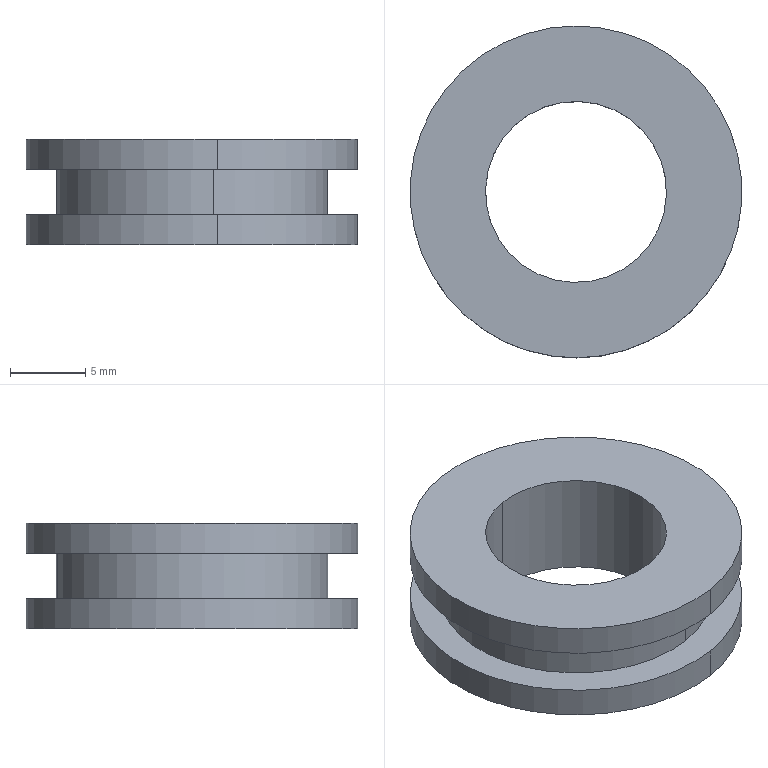Part | SolidWorks | features BaseBody 1 | 1 solid | 12 faces | box 22.001 x 22 x 7.003 mm | volume 1492 mm3 | cylinder 8 | plane 4 | commonest cylinder face diameters 22 x4 12 x2 18 x2
STEP:
#1=CARTESIAN_POINT('',(416.566,223.384,18.485));
#2=VERTEX_POINT('',#1);
#3=CARTESIAN_POINT('',(419.971,201.649,18.486));
#4=VERTEX_POINT('',#3);
#5=CARTESIAN_POINT('',(418.268,212.516,18.486));
#6=DIRECTION('',(0.0001435,0.000000521,-1.));
#7=DIRECTION('',(-0.1548,0.988,-0.00002169));
#8=AXIS2_PLACEMENT_3D('',#5,#6,#7);
#9=CIRCLE('',#8,11.);
#10=EDGE_CURVE('',#2,#4,#9,.T.);
#11=ORIENTED_EDGE('',*,*,#10,.F.);
#12=CARTESIAN_POINT('',(416.565,223.384,20.485));
#13=VERTEX_POINT('',#12);
#14=CARTESIAN_POINT('',(416.566,223.384,13.485));
#15=DIRECTION('',(-0.0001435,-0.000000521,1.));
#16=VECTOR('',#15,1000.);
#17=LINE('',#14,#16);
#18=EDGE_CURVE('',#2,#13,#17,.T.);
#19=ORIENTED_EDGE('',*,*,#18,.T.);
#20=CARTESIAN_POINT('',(419.97,201.649,20.486));
#21=VERTEX_POINT('',#20);
#22=CARTESIAN_POINT('',(418.268,212.516,20.486));
#23=DIRECTION('',(-0.0001435,-0.000000521,1.));
#24=DIRECTION('',(0.1548,-0.988,0.00002169));
#25=AXIS2_PLACEMENT_3D('',#22,#23,#24);
#26=CIRCLE('',#25,11.);
#27=EDGE_CURVE('',#21,#13,#26,.T.);
#28=ORIENTED_EDGE('',*,*,#27,.F.);
#29=CARTESIAN_POINT('',(419.971,201.649,13.486));
#30=DIRECTION('',(-0.0001435,-0.000000521,1.));
#31=VECTOR('',#30,1000.);
#32=LINE('',#29,#31);
#33=EDGE_CURVE('',#4,#21,#32,.T.);
#34=ORIENTED_EDGE('',*,*,#33,.F.);
#35=EDGE_LOOP('',(#11,#19,#28,#34));
#36=FACE_OUTER_BOUND('',#35,.T.);
#37=CARTESIAN_POINT('',(418.269,212.516,13.486));
#38=DIRECTION('',(-0.0001435,-0.000000521,1.));
#39=DIRECTION('',(0.1548,-0.988,0.00002169));
#40=AXIS2_PLACEMENT_3D('',#37,#38,#39);
#41=CYLINDRICAL_SURFACE('',#40,11.);
#42=ADVANCED_FACE('',(#36),#41,.T.);
#43=CARTESIAN_POINT('',(419.661,203.625,18.486));
#44=VERTEX_POINT('',#43);
#45=CARTESIAN_POINT('',(416.875,221.408,18.485));
#46=VERTEX_POINT('',#45);
#47=CARTESIAN_POINT('',(418.268,212.516,18.486));
#48=DIRECTION('',(-0.0001435,-0.000000521,1.));
#49=DIRECTION('',(0.1548,-0.988,0.00002169));
#50=AXIS2_PLACEMENT_3D('',#47,#48,#49);
#51=CIRCLE('',#50,9.);
#52=EDGE_CURVE('',#44,#46,#51,.T.);
#53=ORIENTED_EDGE('',*,*,#52,.F.);
#54=CARTESIAN_POINT('',(419.662,203.625,15.486));
#55=VERTEX_POINT('',#54);
#56=CARTESIAN_POINT('',(419.661,203.625,19.486));
#57=DIRECTION('',(0.0001435,0.000000521,-1.));
#58=VECTOR('',#57,1000.);
#59=LINE('',#56,#58);
#60=EDGE_CURVE('',#44,#55,#59,.T.);
#61=ORIENTED_EDGE('',*,*,#60,.T.);
#62=CARTESIAN_POINT('',(416.876,221.408,15.485));
#63=VERTEX_POINT('',#62);
#64=CARTESIAN_POINT('',(418.269,212.516,15.486));
#65=DIRECTION('',(0.0001435,0.000000521,-1.));
#66=DIRECTION('',(0.1548,-0.988,0.00002169));
#67=AXIS2_PLACEMENT_3D('',#64,#65,#66);
#68=CIRCLE('',#67,9.);
#69=EDGE_CURVE('',#63,#55,#68,.T.);
#70=ORIENTED_EDGE('',*,*,#69,.F.);
#71=CARTESIAN_POINT('',(416.875,221.408,19.485));
#72=DIRECTION('',(0.0001435,0.000000521,-1.));
#73=VECTOR('',#72,1000.);
#74=LINE('',#71,#73);
#75=EDGE_CURVE('',#46,#63,#74,.T.);
#76=ORIENTED_EDGE('',*,*,#75,.F.);
#77=EDGE_LOOP('',(#53,#61,#70,#76));
#78=FACE_OUTER_BOUND('',#77,.T.);
#79=CARTESIAN_POINT('',(418.268,212.516,19.486));
#80=DIRECTION('',(0.0001435,0.000000521,-1.));
#81=DIRECTION('',(-0.1548,0.988,-0.00002169));
#82=AXIS2_PLACEMENT_3D('',#79,#80,#81);
#83=CYLINDRICAL_SURFACE('',#82,9.);
#84=ADVANCED_FACE('',(#78),#83,.T.);
#85=CARTESIAN_POINT('',(416.566,223.384,13.485));
#86=VERTEX_POINT('',#85);
#87=CARTESIAN_POINT('',(419.971,201.649,13.486));
#88=VERTEX_POINT('',#87);
#89=CARTESIAN_POINT('',(418.269,212.516,13.486));
#90=DIRECTION('',(0.0001435,0.000000521,-1.));
#91=DIRECTION('',(1.,0.,0.0001435));
#92=AXIS2_PLACEMENT_3D('',#89,#90,#91);
#93=CIRCLE('',#92,11.);
#94=EDGE_CURVE('',#86,#88,#93,.T.);
#95=ORIENTED_EDGE('',*,*,#94,.F.);
#96=CARTESIAN_POINT('',(416.566,223.384,15.485));
#97=VERTEX_POINT('',#96);
#98=CARTESIAN_POINT('',(416.566,223.384,13.485));
#99=DIRECTION('',(-0.0001435,-0.000000521,1.));
#100=VECTOR('',#99,1000.);
#101=LINE('',#98,#100);
#102=EDGE_CURVE('',#86,#97,#101,.T.);
#103=ORIENTED_EDGE('',*,*,#102,.T.);
#104=CARTESIAN_POINT('',(419.971,201.649,15.486));
#105=VERTEX_POINT('',#104);
#106=CARTESIAN_POINT('',(418.269,212.516,15.486));
#107=DIRECTION('',(-0.0001435,-0.000000521,1.));
#108=DIRECTION('',(-0.1548,0.988,-0.00002169));
#109=AXIS2_PLACEMENT_3D('',#106,#107,#108);
#110=CIRCLE('',#109,11.);
#111=EDGE_CURVE('',#105,#97,#110,.T.);
#112=ORIENTED_EDGE('',*,*,#111,.F.);
#113=CARTESIAN_POINT('',(419.971,201.649,13.486));
#114=DIRECTION('',(-0.0001435,-0.000000521,1.));
#115=VECTOR('',#114,1000.);
#116=LINE('',#113,#115);
#117=EDGE_CURVE('',#88,#105,#116,.T.);
#118=ORIENTED_EDGE('',*,*,#117,.F.);
#119=EDGE_LOOP('',(#95,#103,#112,#118));
#120=FACE_OUTER_BOUND('',#119,.T.);
#121=CARTESIAN_POINT('',(418.269,212.516,13.486));
#122=DIRECTION('',(-0.0001435,-0.000000521,1.));
#123=DIRECTION('',(0.1548,-0.988,0.00002169));
#124=AXIS2_PLACEMENT_3D('',#121,#122,#123);
#125=CYLINDRICAL_SURFACE('',#124,11.);
#126=ADVANCED_FACE('',(#120),#125,.T.);
#127=CARTESIAN_POINT('',(419.196,206.589,20.486));
#128=VERTEX_POINT('',#127);
#129=CARTESIAN_POINT('',(417.339,218.444,20.485));
#130=VERTEX_POINT('',#129);
#131=CARTESIAN_POINT('',(418.268,212.516,20.486));
#132=DIRECTION('',(0.0001435,0.000000521,-1.));
#133=DIRECTION('',(-1.,0.,-0.0001435));
#134=AXIS2_PLACEMENT_3D('',#131,#132,#133);
#135=CIRCLE('',#134,6.);
#136=EDGE_CURVE('',#128,#130,#135,.T.);
#137=ORIENTED_EDGE('',*,*,#136,.F.);
#138=CARTESIAN_POINT('',(419.197,206.589,13.486));
#139=VERTEX_POINT('',#138);
#140=CARTESIAN_POINT('',(419.197,206.589,19.486));
#141=DIRECTION('',(0.0001435,0.000000521,-1.));
#142=VECTOR('',#141,1000.);
#143=LINE('',#140,#142);
#144=EDGE_CURVE('',#128,#139,#143,.T.);
#145=ORIENTED_EDGE('',*,*,#144,.T.);
#146=CARTESIAN_POINT('',(417.34,218.444,13.485));
#147=VERTEX_POINT('',#146);
#148=CARTESIAN_POINT('',(418.269,212.516,13.486));
#149=DIRECTION('',(-0.0001435,-0.000000521,1.));
#150=DIRECTION('',(0.1548,-0.988,0.00002169));
#151=AXIS2_PLACEMENT_3D('',#148,#149,#150);
#152=CIRCLE('',#151,6.);
#153=EDGE_CURVE('',#147,#139,#152,.T.);
#154=ORIENTED_EDGE('',*,*,#153,.F.);
#155=CARTESIAN_POINT('',(417.339,218.444,19.485));
#156=DIRECTION('',(0.0001435,0.000000521,-1.));
#157=VECTOR('',#156,1000.);
#158=LINE('',#155,#157);
#159=EDGE_CURVE('',#130,#147,#158,.T.);
#160=ORIENTED_EDGE('',*,*,#159,.F.);
#161=EDGE_LOOP('',(#137,#145,#154,#160));
#162=FACE_OUTER_BOUND('',#161,.T.);
#163=CARTESIAN_POINT('',(418.268,212.516,19.486));
#164=DIRECTION('',(0.0001435,0.000000521,-1.));
#165=DIRECTION('',(-0.1548,0.988,-0.00002169));
#166=AXIS2_PLACEMENT_3D('',#163,#164,#165);
#167=CYLINDRICAL_SURFACE('',#166,6.);
#168=ADVANCED_FACE('',(#162),#167,.F.);
#169=CARTESIAN_POINT('',(418.268,212.516,20.486));
#170=DIRECTION('',(0.0001435,0.000000521,-1.));
#171=DIRECTION('',(-1.,0.,-0.0001435));
#172=AXIS2_PLACEMENT_3D('',#169,#170,#171);
#173=CIRCLE('',#172,6.);
#174=EDGE_CURVE('',#130,#128,#173,.T.);
#175=ORIENTED_EDGE('',*,*,#174,.T.);
#176=ORIENTED_EDGE('',*,*,#136,.T.);
#177=EDGE_LOOP('',(#175,#176));
#178=FACE_BOUND('',#177,.T.);
#179=ORIENTED_EDGE('',*,*,#27,.T.);
#180=CARTESIAN_POINT('',(418.268,212.516,20.486));
#181=DIRECTION('',(-0.0001435,-0.000000521,1.));
#182=DIRECTION('',(0.1548,-0.988,0.00002169));
#183=AXIS2_PLACEMENT_3D('',#180,#181,#182);
#184=CIRCLE('',#183,11.);
#185=EDGE_CURVE('',#13,#21,#184,.T.);
#186=ORIENTED_EDGE('',*,*,#185,.T.);
#187=EDGE_LOOP('',(#179,#186));
#188=FACE_OUTER_BOUND('',#187,.T.);
#189=CARTESIAN_POINT('',(418.268,212.516,20.486));
#190=DIRECTION('',(-0.0001435,-0.000000521,1.));
#191=DIRECTION('',(-0.003633,1.,0.));
#192=AXIS2_PLACEMENT_3D('',#189,#190,#191);
#193=PLANE('',#192);
#194=ADVANCED_FACE('',(#178,#188),#193,.T.);
#195=ORIENTED_EDGE('',*,*,#144,.F.);
#196=ORIENTED_EDGE('',*,*,#174,.F.);
#197=ORIENTED_EDGE('',*,*,#159,.T.);
#198=CARTESIAN_POINT('',(418.269,212.516,13.486));
#199=DIRECTION('',(-0.0001435,-0.000000521,1.));
#200=DIRECTION('',(0.1548,-0.988,0.00002169));
#201=AXIS2_PLACEMENT_3D('',#198,#199,#200);
#202=CIRCLE('',#201,6.);
#203=EDGE_CURVE('',#139,#147,#202,.T.);
#204=ORIENTED_EDGE('',*,*,#203,.F.);
#205=EDGE_LOOP('',(#195,#196,#197,#204));
#206=FACE_OUTER_BOUND('',#205,.T.);
#207=CARTESIAN_POINT('',(418.268,212.516,19.486));
#208=DIRECTION('',(0.0001435,0.000000521,-1.));
#209=DIRECTION('',(-0.1548,0.988,-0.00002169));
#210=AXIS2_PLACEMENT_3D('',#207,#208,#209);
#211=CYLINDRICAL_SURFACE('',#210,6.);
#212=ADVANCED_FACE('',(#206),#211,.F.);
#213=ORIENTED_EDGE('',*,*,#153,.T.);
#214=ORIENTED_EDGE('',*,*,#203,.T.);
#215=EDGE_LOOP('',(#213,#214));
#216=FACE_BOUND('',#215,.T.);
#217=CARTESIAN_POINT('',(418.269,212.516,13.486));
#218=DIRECTION('',(0.0001435,0.000000521,-1.));
#219=DIRECTION('',(1.,0.,0.0001435));
#220=AXIS2_PLACEMENT_3D('',#217,#218,#219);
#221=CIRCLE('',#220,11.);
#222=EDGE_CURVE('',#88,#86,#221,.T.);
#223=ORIENTED_EDGE('',*,*,#222,.T.);
#224=ORIENTED_EDGE('',*,*,#94,.T.);
#225=EDGE_LOOP('',(#223,#224));
#226=FACE_OUTER_BOUND('',#225,.T.);
#227=CARTESIAN_POINT('',(418.269,212.516,13.486));
#228=DIRECTION('',(0.0001435,0.000000521,-1.));
#229=DIRECTION('',(0.,-1.,-0.000000521));
#230=AXIS2_PLACEMENT_3D('',#227,#228,#229);
#231=PLANE('',#230);
#232=ADVANCED_FACE('',(#216,#226),#231,.T.);
#233=ORIENTED_EDGE('',*,*,#102,.F.);
#234=ORIENTED_EDGE('',*,*,#222,.F.);
#235=ORIENTED_EDGE('',*,*,#117,.T.);
#236=CARTESIAN_POINT('',(418.269,212.516,15.486));
#237=DIRECTION('',(-0.0001435,-0.000000521,1.));
#238=DIRECTION('',(-0.1548,0.988,-0.00002169));
#239=AXIS2_PLACEMENT_3D('',#236,#237,#238);
#240=CIRCLE('',#239,11.);
#241=EDGE_CURVE('',#97,#105,#240,.T.);
#242=ORIENTED_EDGE('',*,*,#241,.F.);
#243=EDGE_LOOP('',(#233,#234,#235,#242));
#244=FACE_OUTER_BOUND('',#243,.T.);
#245=CARTESIAN_POINT('',(418.269,212.516,13.486));
#246=DIRECTION('',(-0.0001435,-0.000000521,1.));
#247=DIRECTION('',(0.1548,-0.988,0.00002169));
#248=AXIS2_PLACEMENT_3D('',#245,#246,#247);
#249=CYLINDRICAL_SURFACE('',#248,11.);
#250=ADVANCED_FACE('',(#244),#249,.T.);
#251=ORIENTED_EDGE('',*,*,#69,.T.);
#252=CARTESIAN_POINT('',(418.269,212.516,15.486));
#253=DIRECTION('',(0.0001435,0.000000521,-1.));
#254=DIRECTION('',(0.1548,-0.988,0.00002169));
#255=AXIS2_PLACEMENT_3D('',#252,#253,#254);
#256=CIRCLE('',#255,9.);
#257=EDGE_CURVE('',#55,#63,#256,.T.);
#258=ORIENTED_EDGE('',*,*,#257,.T.);
#259=EDGE_LOOP('',(#251,#258));
#260=FACE_BOUND('',#259,.T.);
#261=ORIENTED_EDGE('',*,*,#111,.T.);
#262=ORIENTED_EDGE('',*,*,#241,.T.);
#263=EDGE_LOOP('',(#261,#262));
#264=FACE_OUTER_BOUND('',#263,.T.);
#265=CARTESIAN_POINT('',(418.269,212.516,15.486));
#266=DIRECTION('',(0.0001435,0.000000521,-1.));
#267=DIRECTION('',(0.,-1.,-0.000000521));
#268=AXIS2_PLACEMENT_3D('',#265,#266,#267);
#269=PLANE('',#268);
#270=ADVANCED_FACE('',(#260,#264),#269,.F.);
#271=ORIENTED_EDGE('',*,*,#60,.F.);
#272=CARTESIAN_POINT('',(418.268,212.516,18.486));
#273=DIRECTION('',(-0.0001435,-0.000000521,1.));
#274=DIRECTION('',(0.1548,-0.988,0.00002169));
#275=AXIS2_PLACEMENT_3D('',#272,#273,#274);
#276=CIRCLE('',#275,9.);
#277=EDGE_CURVE('',#46,#44,#276,.T.);
#278=ORIENTED_EDGE('',*,*,#277,.F.);
#279=ORIENTED_EDGE('',*,*,#75,.T.);
#280=ORIENTED_EDGE('',*,*,#257,.F.);
#281=EDGE_LOOP('',(#271,#278,#279,#280));
#282=FACE_OUTER_BOUND('',#281,.T.);
#283=CARTESIAN_POINT('',(418.268,212.516,19.486));
#284=DIRECTION('',(0.0001435,0.000000521,-1.));
#285=DIRECTION('',(-0.1548,0.988,-0.00002169));
#286=AXIS2_PLACEMENT_3D('',#283,#284,#285);
#287=CYLINDRICAL_SURFACE('',#286,9.);
#288=ADVANCED_FACE('',(#282),#287,.T.);
#289=ORIENTED_EDGE('',*,*,#277,.T.);
#290=ORIENTED_EDGE('',*,*,#52,.T.);
#291=EDGE_LOOP('',(#289,#290));
#292=FACE_BOUND('',#291,.T.);
#293=CARTESIAN_POINT('',(418.268,212.516,18.486));
#294=DIRECTION('',(0.0001435,0.000000521,-1.));
#295=DIRECTION('',(-0.1548,0.988,-0.00002169));
#296=AXIS2_PLACEMENT_3D('',#293,#294,#295);
#297=CIRCLE('',#296,11.);
#298=EDGE_CURVE('',#4,#2,#297,.T.);
#299=ORIENTED_EDGE('',*,*,#298,.T.);
#300=ORIENTED_EDGE('',*,*,#10,.T.);
#301=EDGE_LOOP('',(#299,#300));
#302=FACE_OUTER_BOUND('',#301,.T.);
#303=CARTESIAN_POINT('',(418.268,212.516,18.486));
#304=DIRECTION('',(-0.0001435,-0.000000521,1.));
#305=DIRECTION('',(-0.003633,1.,0.));
#306=AXIS2_PLACEMENT_3D('',#303,#304,#305);
#307=PLANE('',#306);
#308=ADVANCED_FACE('',(#292,#302),#307,.F.);
#309=ORIENTED_EDGE('',*,*,#18,.F.);
#310=ORIENTED_EDGE('',*,*,#298,.F.);
#311=ORIENTED_EDGE('',*,*,#33,.T.);
#312=ORIENTED_EDGE('',*,*,#185,.F.);
#313=EDGE_LOOP('',(#309,#310,#311,#312));
#314=FACE_OUTER_BOUND('',#313,.T.);
#315=CARTESIAN_POINT('',(418.269,212.516,13.486));
#316=DIRECTION('',(-0.0001435,-0.000000521,1.));
#317=DIRECTION('',(0.1548,-0.988,0.00002169));
#318=AXIS2_PLACEMENT_3D('',#315,#316,#317);
#319=CYLINDRICAL_SURFACE('',#318,11.);
#320=ADVANCED_FACE('',(#314),#319,.T.);
#321=CLOSED_SHELL('',(#42,#84,#126,#168,#194,#212,#232,#250,#270,#288,#308,#320));
#322=MANIFOLD_SOLID_BREP('',#321);
#323=CARTESIAN_POINT('',(0.,0.,0.));
#324=DIRECTION('',(0.,0.,1.));
#325=DIRECTION('',(1.,0.,0.));
#326=AXIS2_PLACEMENT_3D('',#323,#324,#325);
#327=(LENGTH_UNIT()NAMED_UNIT(*)SI_UNIT(.MILLI.,.METRE.));
#328=UNCERTAINTY_MEASURE_WITH_UNIT(LENGTH_MEASURE(0.00001),#327,'','');
#329=(NAMED_UNIT(*)PLANE_ANGLE_UNIT()SI_UNIT($,.RADIAN.));
#330=(NAMED_UNIT(*)SI_UNIT($,.STERADIAN.)SOLID_ANGLE_UNIT());
#331=(GEOMETRIC_REPRESENTATION_CONTEXT(3)GLOBAL_UNCERTAINTY_ASSIGNED_CONTEXT((#328))GLOBAL_UNIT_ASSIGNED_CONTEXT((#327,#329,#330))REPRESENTATION_CONTEXT('',''));
#332=ADVANCED_BREP_SHAPE_REPRESENTATION('',(#322,#326),#331);